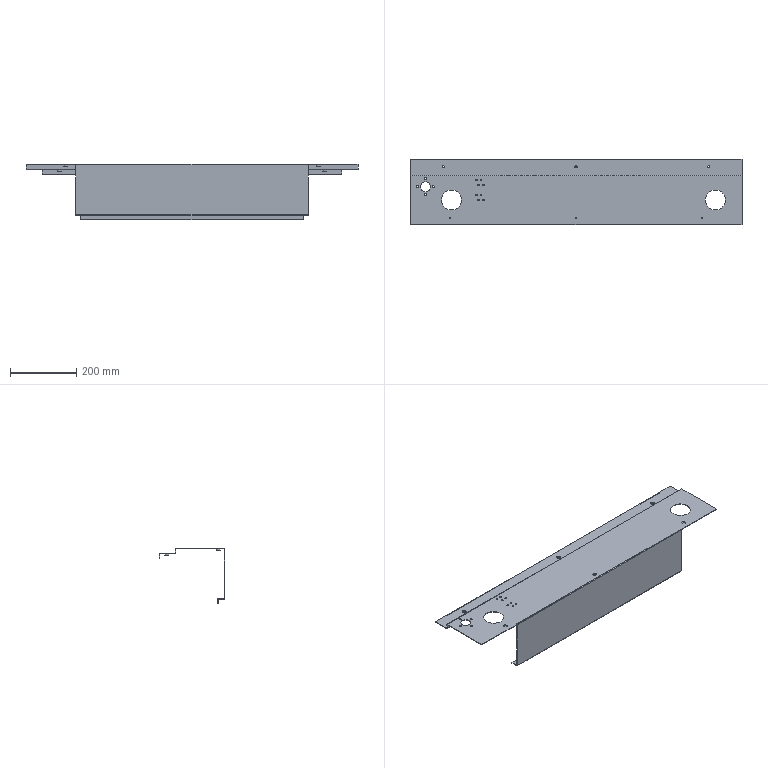Part | STEP file | FHD-021-001-B rack welded part B | 1 solid | 90 faces | box 1000 x 198.5 x 167.5 mm | volume 523284 mm3 | plane 48 | cylinder 42 | commonest cylinder face diameters 5 x8 0.4 x6 3.4 x6 6 x4 4.2 x3 6.8 x3